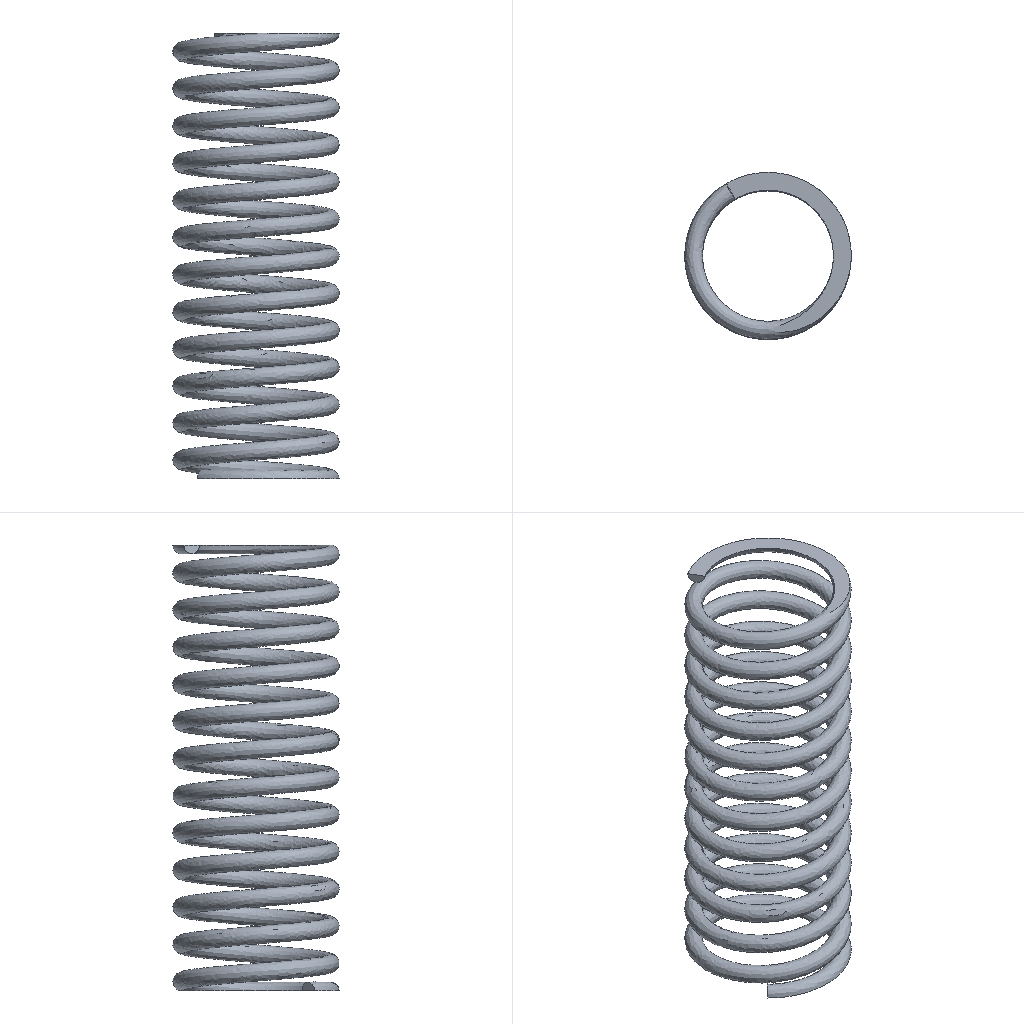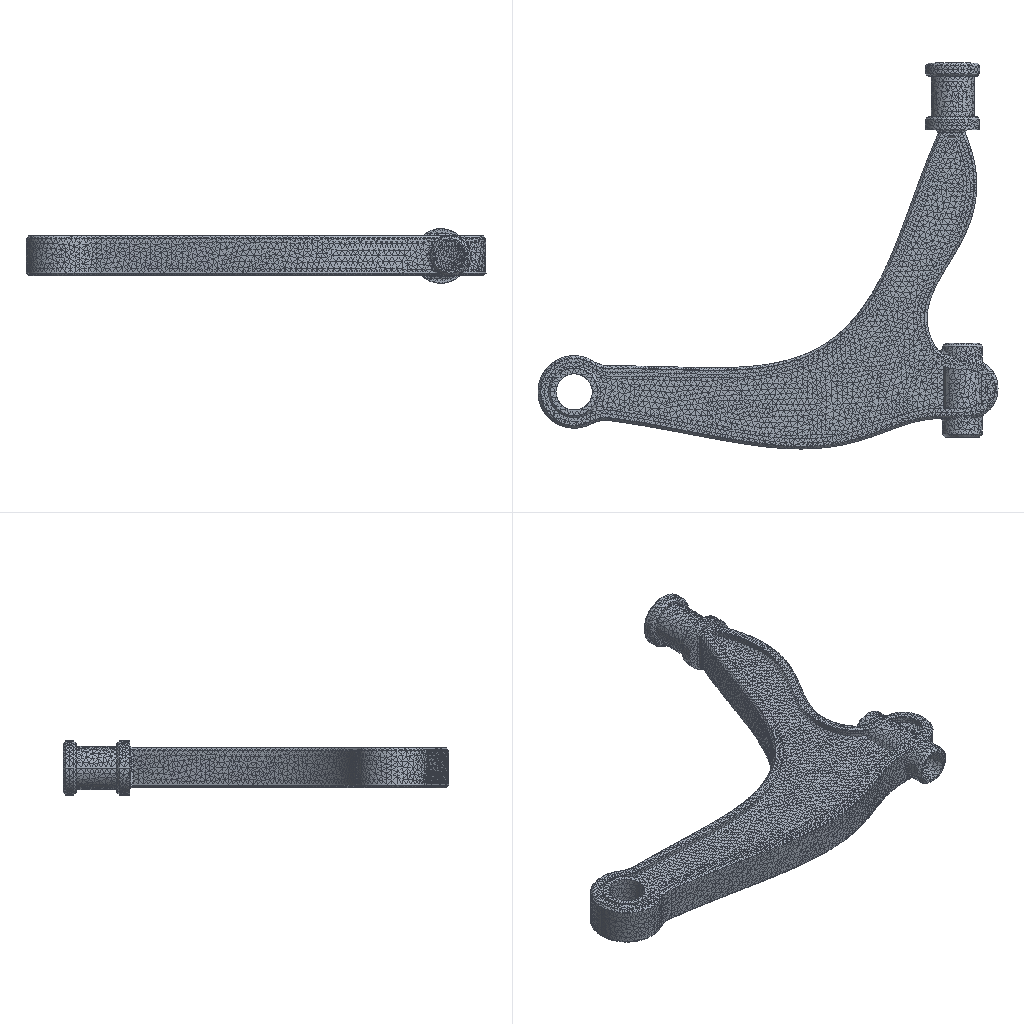Simulation study | ansys workbench
Set-up summary:
category,name,step,type,value,unit,region
solver,ansys_workbench
units,mm-N-s-tonne (MPa),,stated,"/units,MPA"
analysis,deck-1/LS1,,modal,method=lanb; n_modes=10
load_step,deck-1/LS1,deck-1/LS1,modal
analysis,deck-2/LS1,,modal,method=lanb; n_modes=10
load_step,deck-2/LS1,deck-2/LS1,modal
mesh,deck-1.dat,,nodes,226560
mesh,deck-1.dat,,elements,139352
element_type,SOLID187,,,139352,,deck-1.dat
mesh,deck-2.dat,,nodes,144740
mesh,deck-2.dat,,elements,92956
element_type,SOLID187,,,92956,,deck-2.dat
material,?,,E,2.06e+11,Pa
material,?,,nu,0.3
material,?,,density,7850,kg m^-3
material,?,,E,210000,tonne s^-2 mm^-1
material,?,,nu,0.3
material,?,,density,7.85e-09,tonne mm^-3
Results summary:
result,analyses[0].index,,,1
result,analyses[0].system,,,SYS
result,analyses[0].deck,,,deck-1.dat
result,analyses[0].solve_status,,,completed
result,analyses[0].analysis_type,,,modal
result,analyses[0].physics,,,mechanical
result,analyses[0].unit_system,,,"MKS: m, kg, N, s, V, A, degC"
result,analyses[0].n_sets,,,10
result,analyses[0].modal_frequencies_hz[1],,,0
result,analyses[0].modal_frequencies_hz[2],,,0
result,analyses[0].modal_frequencies_hz[3],,,0.0005165
result,analyses[0].modal_frequencies_hz[4],,,0.000825
result,analyses[0].modal_frequencies_hz[5],,,0.00151
result,analyses[0].modal_frequencies_hz[6],,,0.001741
result,analyses[0].modal_frequencies_hz[7],,,32.468
result,analyses[0].modal_frequencies_hz[8],,,32.697
result,analyses[0].modal_frequencies_hz[9],,,34.871
result,analyses[0].modal_frequencies_hz[10],,,39.506
result,analyses[1].index,,,2
result,analyses[1].system,,,SYS-1
result,analyses[1].deck,,,deck-2.dat
result,analyses[1].solve_status,,,completed
result,analyses[1].analysis_type,,,modal
result,analyses[1].physics,,,mechanical
result,analyses[1].unit_system,,,"NMM: mm, ton, N, s, mV, mA, degC"
result,analyses[1].n_sets,,,10
result,analyses[1].modal_frequencies_hz[1],,,0
result,analyses[1].modal_frequencies_hz[2],,,0
result,analyses[1].modal_frequencies_hz[3],,,0
result,analyses[1].modal_frequencies_hz[4],,,0.003578
result,analyses[1].modal_frequencies_hz[5],,,0.004408
result,analyses[1].modal_frequencies_hz[6],,,0.005428
result,analyses[1].modal_frequencies_hz[7],,,2073.17
result,analyses[1].modal_frequencies_hz[8],,,2137.58
result,analyses[1].modal_frequencies_hz[9],,,2389.79
result,analyses[1].modal_frequencies_hz[10],,,3954
result,geometry_export[0][0],,,1.step
result,geometry_export[0][1],,,ok
result,geometry_export[0][2],,,1
result,geometry_export[1][0],,,2.step
result,geometry_export[1][1],,,ok
result,geometry_export[1][2],,,1